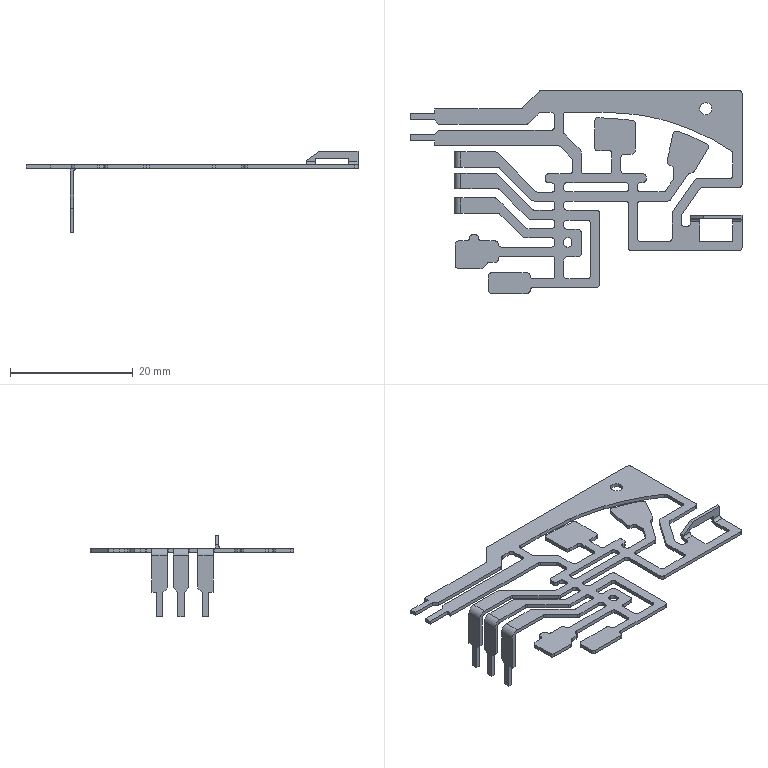Part | NX | features BREP 1 | 1 solid | 285 faces | box 54.103 x 33.1 x 13.3 mm | volume 492.87 mm3 | plane 154 | cylinder 131 | commonest cylinder face diameters 1 x120 2.2 x5 2 x1 69.173 x1 72.496 x1 72.701 x1